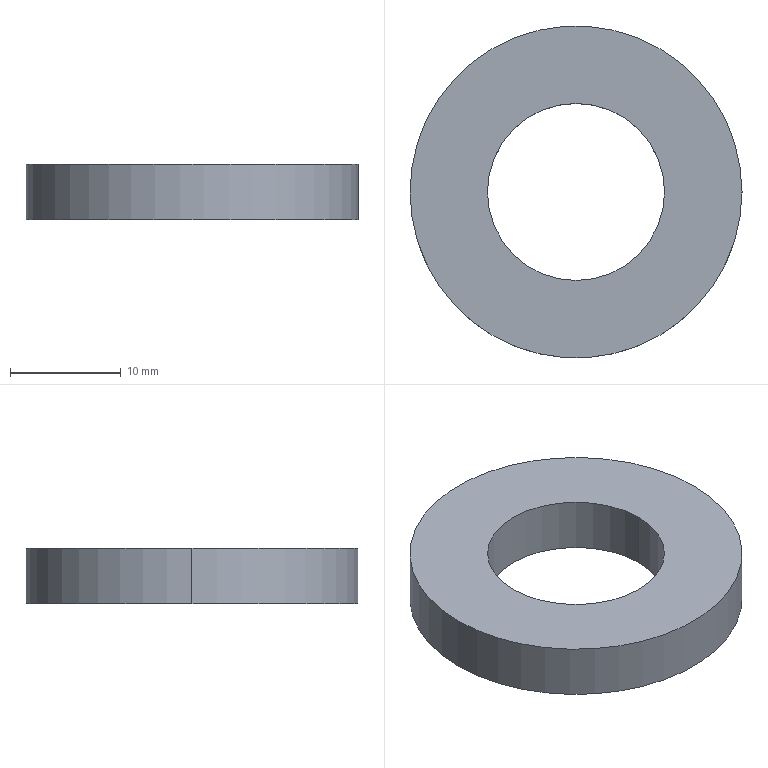Part | STEP file | JAZDQ-D30-d16-T5 polyurethane washer | 1 solid | 6 faces | box 30 x 30 x 5 mm | volume 2529 mm3 | cylinder 4 | plane 2 | commonest cylinder face diameters 16 x2 30 x2
STEP:
#1=CARTESIAN_POINT('',(0.,0.,0.));
#2=DIRECTION('',(0.,0.,1.));
#3=DIRECTION('',(1.,0.,0.));
#4=AXIS2_PLACEMENT_3D('',#1,#2,#3);
#5=CARTESIAN_POINT('',(-8.,0.,2.5));
#6=VERTEX_POINT('',#5);
#7=CARTESIAN_POINT('',(-8.,0.,-2.5));
#8=VERTEX_POINT('',#7);
#9=CARTESIAN_POINT('',(-8.,0.,2.5));
#10=DIRECTION('',(0.,0.,-1.));
#11=VECTOR('',#10,1.);
#12=LINE('',#9,#11);
#13=CARTESIAN_POINT('',(0.,0.,2.5));
#14=DIRECTION('',(0.,0.,-1.));
#15=DIRECTION('',(-1.,0.,0.));
#16=AXIS2_PLACEMENT_3D('',#13,#14,#15);
#17=CYLINDRICAL_SURFACE('',#16,8.);
#18=CARTESIAN_POINT('',(6.283,0.));
#19=DIRECTION('',(0.,1.));
#20=VECTOR('',#19,1.);
#21=LINE('',#18,#20);
#22=(GEOMETRIC_REPRESENTATION_CONTEXT(2)PARAMETRIC_REPRESENTATION_CONTEXT()REPRESENTATION_CONTEXT('',''));
#23=DEFINITIONAL_REPRESENTATION('',(#21),#22);
#24=PCURVE('',#17,#23);
#25=CARTESIAN_POINT('',(0.,0.,2.5));
#26=DIRECTION('',(0.,0.,-1.));
#27=DIRECTION('',(-1.,0.,0.));
#28=AXIS2_PLACEMENT_3D('',#25,#26,#27);
#29=CYLINDRICAL_SURFACE('',#28,8.);
#30=CARTESIAN_POINT('',(0.,0.));
#31=DIRECTION('',(0.,1.));
#32=VECTOR('',#31,1.);
#33=LINE('',#30,#32);
#34=(GEOMETRIC_REPRESENTATION_CONTEXT(2)PARAMETRIC_REPRESENTATION_CONTEXT()REPRESENTATION_CONTEXT('',''));
#35=DEFINITIONAL_REPRESENTATION('',(#33),#34);
#36=PCURVE('',#29,#35);
#37=SURFACE_CURVE('',#12,(#24,#36),.PCURVE_S1.);
#38=EDGE_CURVE('',#6,#8,#37,.T.);
#39=ORIENTED_EDGE('',*,*,#38,.T.);
#40=CARTESIAN_POINT('',(8.,0.,-2.5));
#41=VERTEX_POINT('',#40);
#42=CARTESIAN_POINT('',(0.,0.,-2.5));
#43=DIRECTION('',(0.,0.,1.));
#44=DIRECTION('',(1.,0.,0.));
#45=AXIS2_PLACEMENT_3D('',#42,#43,#44);
#46=CIRCLE('',#45,8.);
#47=CARTESIAN_POINT('',(9.425,5.));
#48=DIRECTION('',(-1.,0.));
#49=VECTOR('',#48,1.);
#50=LINE('',#47,#49);
#51=(GEOMETRIC_REPRESENTATION_CONTEXT(2)PARAMETRIC_REPRESENTATION_CONTEXT()REPRESENTATION_CONTEXT('',''));
#52=DEFINITIONAL_REPRESENTATION('',(#50),#51);
#53=PCURVE('',#17,#52);
#54=CARTESIAN_POINT('',(0.,0.,-2.5));
#55=DIRECTION('',(0.,0.,1.));
#56=DIRECTION('',(1.,0.,0.));
#57=AXIS2_PLACEMENT_3D('',#54,#55,#56);
#58=PLANE('',#57);
#59=CARTESIAN_POINT('',(0.,0.));
#60=DIRECTION('',(1.,0.));
#61=AXIS2_PLACEMENT_2D('',#59,#60);
#62=CIRCLE('',#61,8.);
#63=(GEOMETRIC_REPRESENTATION_CONTEXT(2)PARAMETRIC_REPRESENTATION_CONTEXT()REPRESENTATION_CONTEXT('',''));
#64=DEFINITIONAL_REPRESENTATION('',(#62),#63);
#65=PCURVE('',#58,#64);
#66=SURFACE_CURVE('',#46,(#53,#65),.PCURVE_S1.);
#67=EDGE_CURVE('',#8,#41,#66,.T.);
#68=ORIENTED_EDGE('',*,*,#67,.T.);
#69=CARTESIAN_POINT('',(8.,0.,2.5));
#70=VERTEX_POINT('',#69);
#71=CARTESIAN_POINT('',(8.,0.,2.5));
#72=DIRECTION('',(0.,0.,-1.));
#73=VECTOR('',#72,1.);
#74=LINE('',#71,#73);
#75=CARTESIAN_POINT('',(3.142,0.));
#76=DIRECTION('',(0.,1.));
#77=VECTOR('',#76,1.);
#78=LINE('',#75,#77);
#79=(GEOMETRIC_REPRESENTATION_CONTEXT(2)PARAMETRIC_REPRESENTATION_CONTEXT()REPRESENTATION_CONTEXT('',''));
#80=DEFINITIONAL_REPRESENTATION('',(#78),#79);
#81=PCURVE('',#17,#80);
#82=CARTESIAN_POINT('',(3.142,0.));
#83=DIRECTION('',(0.,1.));
#84=VECTOR('',#83,1.);
#85=LINE('',#82,#84);
#86=(GEOMETRIC_REPRESENTATION_CONTEXT(2)PARAMETRIC_REPRESENTATION_CONTEXT()REPRESENTATION_CONTEXT('',''));
#87=DEFINITIONAL_REPRESENTATION('',(#85),#86);
#88=PCURVE('',#29,#87);
#89=SURFACE_CURVE('',#74,(#81,#88),.PCURVE_S1.);
#90=EDGE_CURVE('',#70,#41,#89,.T.);
#91=ORIENTED_EDGE('',*,*,#90,.F.);
#92=CARTESIAN_POINT('',(0.,0.,2.5));
#93=DIRECTION('',(0.,0.,1.));
#94=DIRECTION('',(1.,0.,0.));
#95=AXIS2_PLACEMENT_3D('',#92,#93,#94);
#96=CIRCLE('',#95,8.);
#97=CARTESIAN_POINT('',(9.425,0.));
#98=DIRECTION('',(-1.,0.));
#99=VECTOR('',#98,1.);
#100=LINE('',#97,#99);
#101=(GEOMETRIC_REPRESENTATION_CONTEXT(2)PARAMETRIC_REPRESENTATION_CONTEXT()REPRESENTATION_CONTEXT('',''));
#102=DEFINITIONAL_REPRESENTATION('',(#100),#101);
#103=PCURVE('',#17,#102);
#104=CARTESIAN_POINT('',(0.,0.,2.5));
#105=DIRECTION('',(0.,0.,1.));
#106=DIRECTION('',(1.,0.,0.));
#107=AXIS2_PLACEMENT_3D('',#104,#105,#106);
#108=PLANE('',#107);
#109=CARTESIAN_POINT('',(0.,0.));
#110=DIRECTION('',(1.,0.));
#111=AXIS2_PLACEMENT_2D('',#109,#110);
#112=CIRCLE('',#111,8.);
#113=(GEOMETRIC_REPRESENTATION_CONTEXT(2)PARAMETRIC_REPRESENTATION_CONTEXT()REPRESENTATION_CONTEXT('',''));
#114=DEFINITIONAL_REPRESENTATION('',(#112),#113);
#115=PCURVE('',#108,#114);
#116=SURFACE_CURVE('',#96,(#103,#115),.PCURVE_S1.);
#117=EDGE_CURVE('',#6,#70,#116,.T.);
#118=ORIENTED_EDGE('',*,*,#117,.F.);
#119=EDGE_LOOP('',(#39,#68,#91,#118));
#120=FACE_BOUND('',#119,.F.);
#121=ADVANCED_FACE('',(#120),#17,.F.);
#122=CARTESIAN_POINT('',(15.,0.,2.5));
#123=VERTEX_POINT('',#122);
#124=CARTESIAN_POINT('',(-15.,0.,2.5));
#125=VERTEX_POINT('',#124);
#126=CARTESIAN_POINT('',(0.,0.,2.5));
#127=DIRECTION('',(0.,0.,1.));
#128=DIRECTION('',(1.,0.,0.));
#129=AXIS2_PLACEMENT_3D('',#126,#127,#128);
#130=CIRCLE('',#129,15.);
#131=CARTESIAN_POINT('',(0.,0.,2.5));
#132=DIRECTION('',(0.,0.,-1.));
#133=DIRECTION('',(-1.,0.,0.));
#134=AXIS2_PLACEMENT_3D('',#131,#132,#133);
#135=CYLINDRICAL_SURFACE('',#134,15.);
#136=CARTESIAN_POINT('',(3.142,0.));
#137=DIRECTION('',(-1.,0.));
#138=VECTOR('',#137,1.);
#139=LINE('',#136,#138);
#140=(GEOMETRIC_REPRESENTATION_CONTEXT(2)PARAMETRIC_REPRESENTATION_CONTEXT()REPRESENTATION_CONTEXT('',''));
#141=DEFINITIONAL_REPRESENTATION('',(#139),#140);
#142=PCURVE('',#135,#141);
#143=CARTESIAN_POINT('',(0.,0.));
#144=DIRECTION('',(1.,0.));
#145=AXIS2_PLACEMENT_2D('',#143,#144);
#146=CIRCLE('',#145,15.);
#147=(GEOMETRIC_REPRESENTATION_CONTEXT(2)PARAMETRIC_REPRESENTATION_CONTEXT()REPRESENTATION_CONTEXT('',''));
#148=DEFINITIONAL_REPRESENTATION('',(#146),#147);
#149=PCURVE('',#108,#148);
#150=SURFACE_CURVE('',#130,(#142,#149),.PCURVE_S1.);
#151=EDGE_CURVE('',#123,#125,#150,.T.);
#152=ORIENTED_EDGE('',*,*,#151,.F.);
#153=CARTESIAN_POINT('',(15.,0.,-2.5));
#154=VERTEX_POINT('',#153);
#155=CARTESIAN_POINT('',(15.,0.,2.5));
#156=DIRECTION('',(0.,0.,-1.));
#157=VECTOR('',#156,1.);
#158=LINE('',#155,#157);
#159=CARTESIAN_POINT('',(3.142,0.));
#160=DIRECTION('',(0.,1.));
#161=VECTOR('',#160,1.);
#162=LINE('',#159,#161);
#163=(GEOMETRIC_REPRESENTATION_CONTEXT(2)PARAMETRIC_REPRESENTATION_CONTEXT()REPRESENTATION_CONTEXT('',''));
#164=DEFINITIONAL_REPRESENTATION('',(#162),#163);
#165=PCURVE('',#135,#164);
#166=CARTESIAN_POINT('',(0.,0.,2.5));
#167=DIRECTION('',(0.,0.,-1.));
#168=DIRECTION('',(-1.,0.,0.));
#169=AXIS2_PLACEMENT_3D('',#166,#167,#168);
#170=CYLINDRICAL_SURFACE('',#169,15.);
#171=CARTESIAN_POINT('',(3.142,0.));
#172=DIRECTION('',(0.,1.));
#173=VECTOR('',#172,1.);
#174=LINE('',#171,#173);
#175=(GEOMETRIC_REPRESENTATION_CONTEXT(2)PARAMETRIC_REPRESENTATION_CONTEXT()REPRESENTATION_CONTEXT('',''));
#176=DEFINITIONAL_REPRESENTATION('',(#174),#175);
#177=PCURVE('',#170,#176);
#178=SURFACE_CURVE('',#158,(#165,#177),.PCURVE_S1.);
#179=EDGE_CURVE('',#123,#154,#178,.T.);
#180=ORIENTED_EDGE('',*,*,#179,.T.);
#181=CARTESIAN_POINT('',(-15.,0.,-2.5));
#182=VERTEX_POINT('',#181);
#183=CARTESIAN_POINT('',(0.,0.,-2.5));
#184=DIRECTION('',(0.,0.,1.));
#185=DIRECTION('',(1.,0.,0.));
#186=AXIS2_PLACEMENT_3D('',#183,#184,#185);
#187=CIRCLE('',#186,15.);
#188=CARTESIAN_POINT('',(3.142,5.));
#189=DIRECTION('',(-1.,0.));
#190=VECTOR('',#189,1.);
#191=LINE('',#188,#190);
#192=(GEOMETRIC_REPRESENTATION_CONTEXT(2)PARAMETRIC_REPRESENTATION_CONTEXT()REPRESENTATION_CONTEXT('',''));
#193=DEFINITIONAL_REPRESENTATION('',(#191),#192);
#194=PCURVE('',#135,#193);
#195=CARTESIAN_POINT('',(0.,0.));
#196=DIRECTION('',(1.,0.));
#197=AXIS2_PLACEMENT_2D('',#195,#196);
#198=CIRCLE('',#197,15.);
#199=(GEOMETRIC_REPRESENTATION_CONTEXT(2)PARAMETRIC_REPRESENTATION_CONTEXT()REPRESENTATION_CONTEXT('',''));
#200=DEFINITIONAL_REPRESENTATION('',(#198),#199);
#201=PCURVE('',#58,#200);
#202=SURFACE_CURVE('',#187,(#194,#201),.PCURVE_S1.);
#203=EDGE_CURVE('',#154,#182,#202,.T.);
#204=ORIENTED_EDGE('',*,*,#203,.T.);
#205=CARTESIAN_POINT('',(-15.,0.,2.5));
#206=DIRECTION('',(0.,0.,-1.));
#207=VECTOR('',#206,1.);
#208=LINE('',#205,#207);
#209=CARTESIAN_POINT('',(0.,0.));
#210=DIRECTION('',(0.,1.));
#211=VECTOR('',#210,1.);
#212=LINE('',#209,#211);
#213=(GEOMETRIC_REPRESENTATION_CONTEXT(2)PARAMETRIC_REPRESENTATION_CONTEXT()REPRESENTATION_CONTEXT('',''));
#214=DEFINITIONAL_REPRESENTATION('',(#212),#213);
#215=PCURVE('',#135,#214);
#216=CARTESIAN_POINT('',(6.283,0.));
#217=DIRECTION('',(0.,1.));
#218=VECTOR('',#217,1.);
#219=LINE('',#216,#218);
#220=(GEOMETRIC_REPRESENTATION_CONTEXT(2)PARAMETRIC_REPRESENTATION_CONTEXT()REPRESENTATION_CONTEXT('',''));
#221=DEFINITIONAL_REPRESENTATION('',(#219),#220);
#222=PCURVE('',#170,#221);
#223=SURFACE_CURVE('',#208,(#215,#222),.PCURVE_S1.);
#224=EDGE_CURVE('',#125,#182,#223,.T.);
#225=ORIENTED_EDGE('',*,*,#224,.F.);
#226=EDGE_LOOP('',(#152,#180,#204,#225));
#227=FACE_BOUND('',#226,.T.);
#228=ADVANCED_FACE('',(#227),#135,.T.);
#229=CARTESIAN_POINT('',(0.,0.,2.5));
#230=DIRECTION('',(0.,0.,1.));
#231=DIRECTION('',(1.,0.,0.));
#232=AXIS2_PLACEMENT_3D('',#229,#230,#231);
#233=CIRCLE('',#232,15.);
#234=CARTESIAN_POINT('',(0.,0.));
#235=DIRECTION('',(1.,0.));
#236=AXIS2_PLACEMENT_2D('',#234,#235);
#237=CIRCLE('',#236,15.);
#238=(GEOMETRIC_REPRESENTATION_CONTEXT(2)PARAMETRIC_REPRESENTATION_CONTEXT()REPRESENTATION_CONTEXT('',''));
#239=DEFINITIONAL_REPRESENTATION('',(#237),#238);
#240=PCURVE('',#108,#239);
#241=CARTESIAN_POINT('',(9.425,0.));
#242=DIRECTION('',(-1.,0.));
#243=VECTOR('',#242,1.);
#244=LINE('',#241,#243);
#245=(GEOMETRIC_REPRESENTATION_CONTEXT(2)PARAMETRIC_REPRESENTATION_CONTEXT()REPRESENTATION_CONTEXT('',''));
#246=DEFINITIONAL_REPRESENTATION('',(#244),#245);
#247=PCURVE('',#170,#246);
#248=SURFACE_CURVE('',#233,(#240,#247),.PCURVE_S1.);
#249=EDGE_CURVE('',#125,#123,#248,.T.);
#250=ORIENTED_EDGE('',*,*,#249,.T.);
#251=ORIENTED_EDGE('',*,*,#151,.T.);
#252=EDGE_LOOP('',(#250,#251));
#253=FACE_BOUND('',#252,.T.);
#254=ORIENTED_EDGE('',*,*,#117,.F.);
#255=CARTESIAN_POINT('',(0.,0.,2.5));
#256=DIRECTION('',(0.,0.,1.));
#257=DIRECTION('',(1.,0.,0.));
#258=AXIS2_PLACEMENT_3D('',#255,#256,#257);
#259=CIRCLE('',#258,8.);
#260=CARTESIAN_POINT('',(0.,0.));
#261=DIRECTION('',(1.,0.));
#262=AXIS2_PLACEMENT_2D('',#260,#261);
#263=CIRCLE('',#262,8.);
#264=(GEOMETRIC_REPRESENTATION_CONTEXT(2)PARAMETRIC_REPRESENTATION_CONTEXT()REPRESENTATION_CONTEXT('',''));
#265=DEFINITIONAL_REPRESENTATION('',(#263),#264);
#266=PCURVE('',#108,#265);
#267=CARTESIAN_POINT('',(3.142,0.));
#268=DIRECTION('',(-1.,0.));
#269=VECTOR('',#268,1.);
#270=LINE('',#267,#269);
#271=(GEOMETRIC_REPRESENTATION_CONTEXT(2)PARAMETRIC_REPRESENTATION_CONTEXT()REPRESENTATION_CONTEXT('',''));
#272=DEFINITIONAL_REPRESENTATION('',(#270),#271);
#273=PCURVE('',#29,#272);
#274=SURFACE_CURVE('',#259,(#266,#273),.PCURVE_S1.);
#275=EDGE_CURVE('',#70,#6,#274,.T.);
#276=ORIENTED_EDGE('',*,*,#275,.F.);
#277=EDGE_LOOP('',(#254,#276));
#278=FACE_BOUND('',#277,.T.);
#279=ADVANCED_FACE('',(#253,#278),#108,.T.);
#280=CARTESIAN_POINT('',(0.,0.,-2.5));
#281=DIRECTION('',(0.,0.,1.));
#282=DIRECTION('',(1.,0.,0.));
#283=AXIS2_PLACEMENT_3D('',#280,#281,#282);
#284=CIRCLE('',#283,15.);
#285=CARTESIAN_POINT('',(0.,0.));
#286=DIRECTION('',(1.,0.));
#287=AXIS2_PLACEMENT_2D('',#285,#286);
#288=CIRCLE('',#287,15.);
#289=(GEOMETRIC_REPRESENTATION_CONTEXT(2)PARAMETRIC_REPRESENTATION_CONTEXT()REPRESENTATION_CONTEXT('',''));
#290=DEFINITIONAL_REPRESENTATION('',(#288),#289);
#291=PCURVE('',#58,#290);
#292=CARTESIAN_POINT('',(9.425,5.));
#293=DIRECTION('',(-1.,0.));
#294=VECTOR('',#293,1.);
#295=LINE('',#292,#294);
#296=(GEOMETRIC_REPRESENTATION_CONTEXT(2)PARAMETRIC_REPRESENTATION_CONTEXT()REPRESENTATION_CONTEXT('',''));
#297=DEFINITIONAL_REPRESENTATION('',(#295),#296);
#298=PCURVE('',#170,#297);
#299=SURFACE_CURVE('',#284,(#291,#298),.PCURVE_S1.);
#300=EDGE_CURVE('',#182,#154,#299,.T.);
#301=ORIENTED_EDGE('',*,*,#300,.F.);
#302=ORIENTED_EDGE('',*,*,#203,.F.);
#303=EDGE_LOOP('',(#301,#302));
#304=FACE_BOUND('',#303,.T.);
#305=ORIENTED_EDGE('',*,*,#67,.T.);
#306=CARTESIAN_POINT('',(0.,0.,-2.5));
#307=DIRECTION('',(0.,0.,1.));
#308=DIRECTION('',(1.,0.,0.));
#309=AXIS2_PLACEMENT_3D('',#306,#307,#308);
#310=CIRCLE('',#309,8.);
#311=CARTESIAN_POINT('',(0.,0.));
#312=DIRECTION('',(1.,0.));
#313=AXIS2_PLACEMENT_2D('',#311,#312);
#314=CIRCLE('',#313,8.);
#315=(GEOMETRIC_REPRESENTATION_CONTEXT(2)PARAMETRIC_REPRESENTATION_CONTEXT()REPRESENTATION_CONTEXT('',''));
#316=DEFINITIONAL_REPRESENTATION('',(#314),#315);
#317=PCURVE('',#58,#316);
#318=CARTESIAN_POINT('',(3.142,5.));
#319=DIRECTION('',(-1.,0.));
#320=VECTOR('',#319,1.);
#321=LINE('',#318,#320);
#322=(GEOMETRIC_REPRESENTATION_CONTEXT(2)PARAMETRIC_REPRESENTATION_CONTEXT()REPRESENTATION_CONTEXT('',''));
#323=DEFINITIONAL_REPRESENTATION('',(#321),#322);
#324=PCURVE('',#29,#323);
#325=SURFACE_CURVE('',#310,(#317,#324),.PCURVE_S1.);
#326=EDGE_CURVE('',#41,#8,#325,.T.);
#327=ORIENTED_EDGE('',*,*,#326,.T.);
#328=EDGE_LOOP('',(#305,#327));
#329=FACE_BOUND('',#328,.T.);
#330=ADVANCED_FACE('',(#304,#329),#58,.F.);
#331=ORIENTED_EDGE('',*,*,#179,.F.);
#332=ORIENTED_EDGE('',*,*,#249,.F.);
#333=ORIENTED_EDGE('',*,*,#224,.T.);
#334=ORIENTED_EDGE('',*,*,#300,.T.);
#335=EDGE_LOOP('',(#331,#332,#333,#334));
#336=FACE_BOUND('',#335,.T.);
#337=ADVANCED_FACE('',(#336),#170,.T.);
#338=ORIENTED_EDGE('',*,*,#326,.T.);
#339=ORIENTED_EDGE('',*,*,#38,.F.);
#340=ORIENTED_EDGE('',*,*,#275,.F.);
#341=ORIENTED_EDGE('',*,*,#90,.T.);
#342=EDGE_LOOP('',(#338,#339,#340,#341));
#343=FACE_BOUND('',#342,.F.);
#344=ADVANCED_FACE('',(#343),#29,.F.);
#345=CLOSED_SHELL('',(#121,#228,#279,#330,#337,#344));
#346=MANIFOLD_SOLID_BREP('',#345);
#347=(LENGTH_UNIT()NAMED_UNIT(*)SI_UNIT(.MILLI.,.METRE.));
#348=UNCERTAINTY_MEASURE_WITH_UNIT(LENGTH_MEASURE(0.0000001),#347,'','');
#349=(NAMED_UNIT(*)PLANE_ANGLE_UNIT()SI_UNIT($,.RADIAN.));
#350=(NAMED_UNIT(*)SI_UNIT($,.STERADIAN.)SOLID_ANGLE_UNIT());
#351=(GEOMETRIC_REPRESENTATION_CONTEXT(3)GLOBAL_UNCERTAINTY_ASSIGNED_CONTEXT((#348))GLOBAL_UNIT_ASSIGNED_CONTEXT((#347,#349,#350))REPRESENTATION_CONTEXT('',''));
#352=ADVANCED_BREP_SHAPE_REPRESENTATION('',(#4,#346),#351);